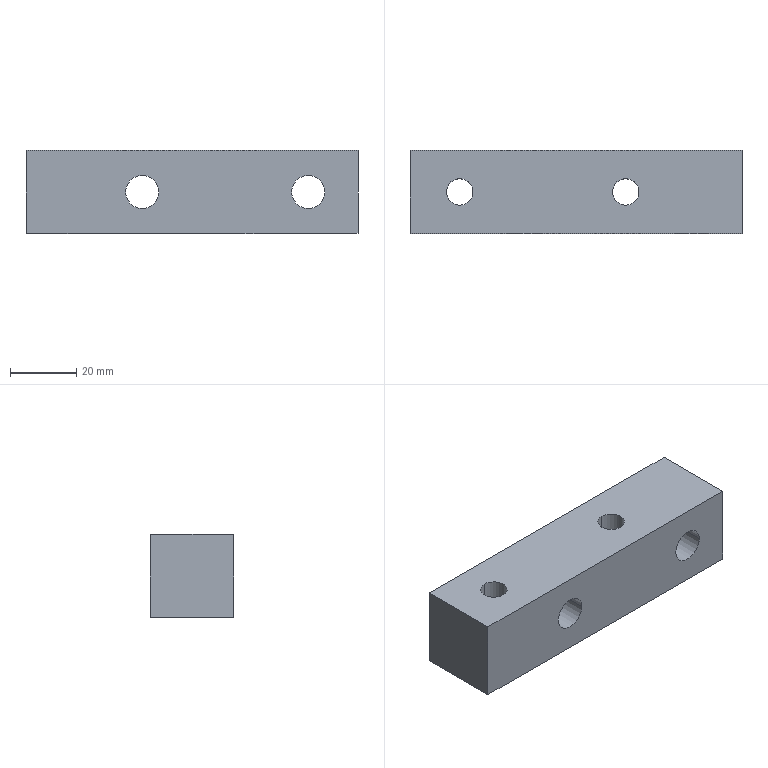Part | STEP file | J453-EBZ05-11-00 | 1 solid | 14 faces | box 100 x 25 x 25 mm | volume 56060 mm3 | cylinder 8 | plane 6 | commonest cylinder face diameters 8 x4 10 x4
STEP:
#1=CARTESIAN_POINT('',(0.,0.,0.));
#2=DIRECTION('',(0.,0.,1.));
#3=DIRECTION('',(1.,0.,0.));
#4=AXIS2_PLACEMENT_3D('',#1,#2,#3);
#5=CARTESIAN_POINT('',(80.,25.,12.5));
#6=VERTEX_POINT('',#5);
#7=CARTESIAN_POINT('',(80.,0.,12.5));
#8=VERTEX_POINT('',#7);
#9=CARTESIAN_POINT('',(80.,25.,12.5));
#10=DIRECTION('',(0.,-1.,0.));
#11=VECTOR('',#10,1.);
#12=LINE('',#9,#11);
#13=CARTESIAN_POINT('',(85.,25.,12.5));
#14=DIRECTION('',(0.,-1.,0.));
#15=DIRECTION('',(-1.,0.,0.));
#16=AXIS2_PLACEMENT_3D('',#13,#14,#15);
#17=CYLINDRICAL_SURFACE('',#16,5.);
#18=CARTESIAN_POINT('',(6.283,0.));
#19=DIRECTION('',(0.,1.));
#20=VECTOR('',#19,1.);
#21=LINE('',#18,#20);
#22=(GEOMETRIC_REPRESENTATION_CONTEXT(2)PARAMETRIC_REPRESENTATION_CONTEXT()REPRESENTATION_CONTEXT('',''));
#23=DEFINITIONAL_REPRESENTATION('',(#21),#22);
#24=PCURVE('',#17,#23);
#25=CARTESIAN_POINT('',(85.,25.,12.5));
#26=DIRECTION('',(0.,-1.,0.));
#27=DIRECTION('',(-1.,0.,0.));
#28=AXIS2_PLACEMENT_3D('',#25,#26,#27);
#29=CYLINDRICAL_SURFACE('',#28,5.);
#30=CARTESIAN_POINT('',(0.,0.));
#31=DIRECTION('',(0.,1.));
#32=VECTOR('',#31,1.);
#33=LINE('',#30,#32);
#34=(GEOMETRIC_REPRESENTATION_CONTEXT(2)PARAMETRIC_REPRESENTATION_CONTEXT()REPRESENTATION_CONTEXT('',''));
#35=DEFINITIONAL_REPRESENTATION('',(#33),#34);
#36=PCURVE('',#29,#35);
#37=SURFACE_CURVE('',#12,(#24,#36),.PCURVE_S1.);
#38=EDGE_CURVE('',#6,#8,#37,.T.);
#39=ORIENTED_EDGE('',*,*,#38,.T.);
#40=CARTESIAN_POINT('',(90.,0.,12.5));
#41=VERTEX_POINT('',#40);
#42=CARTESIAN_POINT('',(85.,0.,12.5));
#43=DIRECTION('',(0.,1.,0.));
#44=DIRECTION('',(1.,0.,0.));
#45=AXIS2_PLACEMENT_3D('',#42,#43,#44);
#46=CIRCLE('',#45,5.);
#47=CARTESIAN_POINT('',(9.425,25.));
#48=DIRECTION('',(-1.,0.));
#49=VECTOR('',#48,1.);
#50=LINE('',#47,#49);
#51=(GEOMETRIC_REPRESENTATION_CONTEXT(2)PARAMETRIC_REPRESENTATION_CONTEXT()REPRESENTATION_CONTEXT('',''));
#52=DEFINITIONAL_REPRESENTATION('',(#50),#51);
#53=PCURVE('',#17,#52);
#54=CARTESIAN_POINT('',(0.,0.,12.5));
#55=DIRECTION('',(0.,-1.,0.));
#56=DIRECTION('',(-1.,0.,0.));
#57=AXIS2_PLACEMENT_3D('',#54,#55,#56);
#58=PLANE('',#57);
#59=CARTESIAN_POINT('',(-90.,0.));
#60=CARTESIAN_POINT('',(-90.,8.66));
#61=CARTESIAN_POINT('',(-82.5,4.33));
#62=CARTESIAN_POINT('',(-75.,0.));
#63=CARTESIAN_POINT('',(-82.5,-4.33));
#64=CARTESIAN_POINT('',(-90.,-8.66));
#65=CARTESIAN_POINT('',(-90.,0.));
#66=(BOUNDED_CURVE()B_SPLINE_CURVE(2,(#59,#60,#61,#62,#63,#64,#65),.UNSPECIFIED.,.T.,.F.)B_SPLINE_CURVE_WITH_KNOTS((1,2,2,2,2,1),(-2.094,0.,2.094,4.189,6.283,8.378),.UNSPECIFIED.)CURVE()GEOMETRIC_REPRESENTATION_ITEM()RATIONAL_B_SPLINE_CURVE((1.,0.5,1.,0.5,1.,0.5,1.))REPRESENTATION_ITEM(''));
#67=(GEOMETRIC_REPRESENTATION_CONTEXT(2)PARAMETRIC_REPRESENTATION_CONTEXT()REPRESENTATION_CONTEXT('',''));
#68=DEFINITIONAL_REPRESENTATION('',(#66),#67);
#69=PCURVE('',#58,#68);
#70=SURFACE_CURVE('',#46,(#53,#69),.PCURVE_S1.);
#71=EDGE_CURVE('',#8,#41,#70,.T.);
#72=ORIENTED_EDGE('',*,*,#71,.T.);
#73=CARTESIAN_POINT('',(90.,25.,12.5));
#74=VERTEX_POINT('',#73);
#75=CARTESIAN_POINT('',(90.,25.,12.5));
#76=DIRECTION('',(0.,-1.,0.));
#77=VECTOR('',#76,1.);
#78=LINE('',#75,#77);
#79=CARTESIAN_POINT('',(3.142,0.));
#80=DIRECTION('',(0.,1.));
#81=VECTOR('',#80,1.);
#82=LINE('',#79,#81);
#83=(GEOMETRIC_REPRESENTATION_CONTEXT(2)PARAMETRIC_REPRESENTATION_CONTEXT()REPRESENTATION_CONTEXT('',''));
#84=DEFINITIONAL_REPRESENTATION('',(#82),#83);
#85=PCURVE('',#17,#84);
#86=CARTESIAN_POINT('',(3.142,0.));
#87=DIRECTION('',(0.,1.));
#88=VECTOR('',#87,1.);
#89=LINE('',#86,#88);
#90=(GEOMETRIC_REPRESENTATION_CONTEXT(2)PARAMETRIC_REPRESENTATION_CONTEXT()REPRESENTATION_CONTEXT('',''));
#91=DEFINITIONAL_REPRESENTATION('',(#89),#90);
#92=PCURVE('',#29,#91);
#93=SURFACE_CURVE('',#78,(#85,#92),.PCURVE_S1.);
#94=EDGE_CURVE('',#74,#41,#93,.T.);
#95=ORIENTED_EDGE('',*,*,#94,.F.);
#96=CARTESIAN_POINT('',(85.,25.,12.5));
#97=DIRECTION('',(0.,-1.,0.));
#98=DIRECTION('',(-1.,0.,0.));
#99=AXIS2_PLACEMENT_3D('',#96,#97,#98);
#100=CIRCLE('',#99,5.);
#101=CARTESIAN_POINT('',(0.,0.));
#102=DIRECTION('',(1.,0.));
#103=VECTOR('',#102,1.);
#104=LINE('',#101,#103);
#105=(GEOMETRIC_REPRESENTATION_CONTEXT(2)PARAMETRIC_REPRESENTATION_CONTEXT()REPRESENTATION_CONTEXT('',''));
#106=DEFINITIONAL_REPRESENTATION('',(#104),#105);
#107=PCURVE('',#17,#106);
#108=CARTESIAN_POINT('',(0.,25.,12.5));
#109=DIRECTION('',(0.,1.,0.));
#110=DIRECTION('',(1.,0.,0.));
#111=AXIS2_PLACEMENT_3D('',#108,#109,#110);
#112=PLANE('',#111);
#113=CARTESIAN_POINT('',(80.,0.));
#114=CARTESIAN_POINT('',(80.,8.66));
#115=CARTESIAN_POINT('',(87.5,4.33));
#116=CARTESIAN_POINT('',(95.,0.));
#117=CARTESIAN_POINT('',(87.5,-4.33));
#118=CARTESIAN_POINT('',(80.,-8.66));
#119=CARTESIAN_POINT('',(80.,0.));
#120=(BOUNDED_CURVE()B_SPLINE_CURVE(2,(#113,#114,#115,#116,#117,#118,#119),.UNSPECIFIED.,.T.,.F.)B_SPLINE_CURVE_WITH_KNOTS((1,2,2,2,2,1),(-2.094,0.,2.094,4.189,6.283,8.378),.UNSPECIFIED.)CURVE()GEOMETRIC_REPRESENTATION_ITEM()RATIONAL_B_SPLINE_CURVE((1.,0.5,1.,0.5,1.,0.5,1.))REPRESENTATION_ITEM(''));
#121=(GEOMETRIC_REPRESENTATION_CONTEXT(2)PARAMETRIC_REPRESENTATION_CONTEXT()REPRESENTATION_CONTEXT('',''));
#122=DEFINITIONAL_REPRESENTATION('',(#120),#121);
#123=PCURVE('',#112,#122);
#124=SURFACE_CURVE('',#100,(#107,#123),.PCURVE_S1.);
#125=EDGE_CURVE('',#74,#6,#124,.T.);
#126=ORIENTED_EDGE('',*,*,#125,.T.);
#127=EDGE_LOOP('',(#39,#72,#95,#126));
#128=FACE_BOUND('',#127,.F.);
#129=ADVANCED_FACE('',(#128),#17,.F.);
#130=CARTESIAN_POINT('',(30.,25.,12.5));
#131=VERTEX_POINT('',#130);
#132=CARTESIAN_POINT('',(30.,0.,12.5));
#133=VERTEX_POINT('',#132);
#134=CARTESIAN_POINT('',(30.,25.,12.5));
#135=DIRECTION('',(0.,-1.,0.));
#136=VECTOR('',#135,1.);
#137=LINE('',#134,#136);
#138=CARTESIAN_POINT('',(35.,25.,12.5));
#139=DIRECTION('',(0.,-1.,0.));
#140=DIRECTION('',(-1.,0.,0.));
#141=AXIS2_PLACEMENT_3D('',#138,#139,#140);
#142=CYLINDRICAL_SURFACE('',#141,5.);
#143=CARTESIAN_POINT('',(6.283,0.));
#144=DIRECTION('',(0.,1.));
#145=VECTOR('',#144,1.);
#146=LINE('',#143,#145);
#147=(GEOMETRIC_REPRESENTATION_CONTEXT(2)PARAMETRIC_REPRESENTATION_CONTEXT()REPRESENTATION_CONTEXT('',''));
#148=DEFINITIONAL_REPRESENTATION('',(#146),#147);
#149=PCURVE('',#142,#148);
#150=CARTESIAN_POINT('',(35.,25.,12.5));
#151=DIRECTION('',(0.,-1.,0.));
#152=DIRECTION('',(-1.,0.,0.));
#153=AXIS2_PLACEMENT_3D('',#150,#151,#152);
#154=CYLINDRICAL_SURFACE('',#153,5.);
#155=CARTESIAN_POINT('',(0.,0.));
#156=DIRECTION('',(0.,1.));
#157=VECTOR('',#156,1.);
#158=LINE('',#155,#157);
#159=(GEOMETRIC_REPRESENTATION_CONTEXT(2)PARAMETRIC_REPRESENTATION_CONTEXT()REPRESENTATION_CONTEXT('',''));
#160=DEFINITIONAL_REPRESENTATION('',(#158),#159);
#161=PCURVE('',#154,#160);
#162=SURFACE_CURVE('',#137,(#149,#161),.PCURVE_S1.);
#163=EDGE_CURVE('',#131,#133,#162,.T.);
#164=ORIENTED_EDGE('',*,*,#163,.T.);
#165=CARTESIAN_POINT('',(40.,0.,12.5));
#166=VERTEX_POINT('',#165);
#167=CARTESIAN_POINT('',(35.,0.,12.5));
#168=DIRECTION('',(0.,1.,0.));
#169=DIRECTION('',(1.,0.,0.));
#170=AXIS2_PLACEMENT_3D('',#167,#168,#169);
#171=CIRCLE('',#170,5.);
#172=CARTESIAN_POINT('',(9.425,25.));
#173=DIRECTION('',(-1.,0.));
#174=VECTOR('',#173,1.);
#175=LINE('',#172,#174);
#176=(GEOMETRIC_REPRESENTATION_CONTEXT(2)PARAMETRIC_REPRESENTATION_CONTEXT()REPRESENTATION_CONTEXT('',''));
#177=DEFINITIONAL_REPRESENTATION('',(#175),#176);
#178=PCURVE('',#142,#177);
#179=CARTESIAN_POINT('',(-40.,0.));
#180=CARTESIAN_POINT('',(-40.,8.66));
#181=CARTESIAN_POINT('',(-32.5,4.33));
#182=CARTESIAN_POINT('',(-25.,0.));
#183=CARTESIAN_POINT('',(-32.5,-4.33));
#184=CARTESIAN_POINT('',(-40.,-8.66));
#185=CARTESIAN_POINT('',(-40.,0.));
#186=(BOUNDED_CURVE()B_SPLINE_CURVE(2,(#179,#180,#181,#182,#183,#184,#185),.UNSPECIFIED.,.T.,.F.)B_SPLINE_CURVE_WITH_KNOTS((1,2,2,2,2,1),(-2.094,0.,2.094,4.189,6.283,8.378),.UNSPECIFIED.)CURVE()GEOMETRIC_REPRESENTATION_ITEM()RATIONAL_B_SPLINE_CURVE((1.,0.5,1.,0.5,1.,0.5,1.))REPRESENTATION_ITEM(''));
#187=(GEOMETRIC_REPRESENTATION_CONTEXT(2)PARAMETRIC_REPRESENTATION_CONTEXT()REPRESENTATION_CONTEXT('',''));
#188=DEFINITIONAL_REPRESENTATION('',(#186),#187);
#189=PCURVE('',#58,#188);
#190=SURFACE_CURVE('',#171,(#178,#189),.PCURVE_S1.);
#191=EDGE_CURVE('',#133,#166,#190,.T.);
#192=ORIENTED_EDGE('',*,*,#191,.T.);
#193=CARTESIAN_POINT('',(40.,25.,12.5));
#194=VERTEX_POINT('',#193);
#195=CARTESIAN_POINT('',(40.,25.,12.5));
#196=DIRECTION('',(0.,-1.,0.));
#197=VECTOR('',#196,1.);
#198=LINE('',#195,#197);
#199=CARTESIAN_POINT('',(3.142,0.));
#200=DIRECTION('',(0.,1.));
#201=VECTOR('',#200,1.);
#202=LINE('',#199,#201);
#203=(GEOMETRIC_REPRESENTATION_CONTEXT(2)PARAMETRIC_REPRESENTATION_CONTEXT()REPRESENTATION_CONTEXT('',''));
#204=DEFINITIONAL_REPRESENTATION('',(#202),#203);
#205=PCURVE('',#142,#204);
#206=CARTESIAN_POINT('',(3.142,0.));
#207=DIRECTION('',(0.,1.));
#208=VECTOR('',#207,1.);
#209=LINE('',#206,#208);
#210=(GEOMETRIC_REPRESENTATION_CONTEXT(2)PARAMETRIC_REPRESENTATION_CONTEXT()REPRESENTATION_CONTEXT('',''));
#211=DEFINITIONAL_REPRESENTATION('',(#209),#210);
#212=PCURVE('',#154,#211);
#213=SURFACE_CURVE('',#198,(#205,#212),.PCURVE_S1.);
#214=EDGE_CURVE('',#194,#166,#213,.T.);
#215=ORIENTED_EDGE('',*,*,#214,.F.);
#216=CARTESIAN_POINT('',(35.,25.,12.5));
#217=DIRECTION('',(0.,-1.,0.));
#218=DIRECTION('',(-1.,0.,0.));
#219=AXIS2_PLACEMENT_3D('',#216,#217,#218);
#220=CIRCLE('',#219,5.);
#221=CARTESIAN_POINT('',(0.,0.));
#222=DIRECTION('',(1.,0.));
#223=VECTOR('',#222,1.);
#224=LINE('',#221,#223);
#225=(GEOMETRIC_REPRESENTATION_CONTEXT(2)PARAMETRIC_REPRESENTATION_CONTEXT()REPRESENTATION_CONTEXT('',''));
#226=DEFINITIONAL_REPRESENTATION('',(#224),#225);
#227=PCURVE('',#142,#226);
#228=CARTESIAN_POINT('',(30.,0.));
#229=CARTESIAN_POINT('',(30.,8.66));
#230=CARTESIAN_POINT('',(37.5,4.33));
#231=CARTESIAN_POINT('',(45.,0.));
#232=CARTESIAN_POINT('',(37.5,-4.33));
#233=CARTESIAN_POINT('',(30.,-8.66));
#234=CARTESIAN_POINT('',(30.,0.));
#235=(BOUNDED_CURVE()B_SPLINE_CURVE(2,(#228,#229,#230,#231,#232,#233,#234),.UNSPECIFIED.,.T.,.F.)B_SPLINE_CURVE_WITH_KNOTS((1,2,2,2,2,1),(-2.094,0.,2.094,4.189,6.283,8.378),.UNSPECIFIED.)CURVE()GEOMETRIC_REPRESENTATION_ITEM()RATIONAL_B_SPLINE_CURVE((1.,0.5,1.,0.5,1.,0.5,1.))REPRESENTATION_ITEM(''));
#236=(GEOMETRIC_REPRESENTATION_CONTEXT(2)PARAMETRIC_REPRESENTATION_CONTEXT()REPRESENTATION_CONTEXT('',''));
#237=DEFINITIONAL_REPRESENTATION('',(#235),#236);
#238=PCURVE('',#112,#237);
#239=SURFACE_CURVE('',#220,(#227,#238),.PCURVE_S1.);
#240=EDGE_CURVE('',#194,#131,#239,.T.);
#241=ORIENTED_EDGE('',*,*,#240,.T.);
#242=EDGE_LOOP('',(#164,#192,#215,#241));
#243=FACE_BOUND('',#242,.F.);
#244=ADVANCED_FACE('',(#243),#142,.F.);
#245=CARTESIAN_POINT('',(65.,8.5,0.));
#246=VERTEX_POINT('',#245);
#247=CARTESIAN_POINT('',(65.,8.5,25.));
#248=VERTEX_POINT('',#247);
#249=CARTESIAN_POINT('',(65.,8.5,0.));
#250=DIRECTION('',(0.,0.,1.));
#251=VECTOR('',#250,1.);
#252=LINE('',#249,#251);
#253=CARTESIAN_POINT('',(65.,12.5,0.));
#254=DIRECTION('',(0.,0.,1.));
#255=DIRECTION('',(0.,-1.,0.));
#256=AXIS2_PLACEMENT_3D('',#253,#254,#255);
#257=CYLINDRICAL_SURFACE('',#256,4.);
#258=CARTESIAN_POINT('',(6.283,0.));
#259=DIRECTION('',(0.,1.));
#260=VECTOR('',#259,1.);
#261=LINE('',#258,#260);
#262=(GEOMETRIC_REPRESENTATION_CONTEXT(2)PARAMETRIC_REPRESENTATION_CONTEXT()REPRESENTATION_CONTEXT('',''));
#263=DEFINITIONAL_REPRESENTATION('',(#261),#262);
#264=PCURVE('',#257,#263);
#265=CARTESIAN_POINT('',(65.,12.5,0.));
#266=DIRECTION('',(0.,0.,1.));
#267=DIRECTION('',(0.,-1.,0.));
#268=AXIS2_PLACEMENT_3D('',#265,#266,#267);
#269=CYLINDRICAL_SURFACE('',#268,4.);
#270=CARTESIAN_POINT('',(0.,0.));
#271=DIRECTION('',(0.,1.));
#272=VECTOR('',#271,1.);
#273=LINE('',#270,#272);
#274=(GEOMETRIC_REPRESENTATION_CONTEXT(2)PARAMETRIC_REPRESENTATION_CONTEXT()REPRESENTATION_CONTEXT('',''));
#275=DEFINITIONAL_REPRESENTATION('',(#273),#274);
#276=PCURVE('',#269,#275);
#277=SURFACE_CURVE('',#252,(#264,#276),.PCURVE_S1.);
#278=EDGE_CURVE('',#246,#248,#277,.T.);
#279=ORIENTED_EDGE('',*,*,#278,.T.);
#280=CARTESIAN_POINT('',(65.,16.5,25.));
#281=VERTEX_POINT('',#280);
#282=CARTESIAN_POINT('',(65.,12.5,25.));
#283=DIRECTION('',(0.,0.,-1.));
#284=DIRECTION('',(0.,1.,0.));
#285=AXIS2_PLACEMENT_3D('',#282,#283,#284);
#286=CIRCLE('',#285,4.);
#287=CARTESIAN_POINT('',(9.425,25.));
#288=DIRECTION('',(-1.,0.));
#289=VECTOR('',#288,1.);
#290=LINE('',#287,#289);
#291=(GEOMETRIC_REPRESENTATION_CONTEXT(2)PARAMETRIC_REPRESENTATION_CONTEXT()REPRESENTATION_CONTEXT('',''));
#292=DEFINITIONAL_REPRESENTATION('',(#290),#291);
#293=PCURVE('',#257,#292);
#294=CARTESIAN_POINT('',(0.,12.5,25.));
#295=DIRECTION('',(0.,0.,1.));
#296=DIRECTION('',(1.,0.,0.));
#297=AXIS2_PLACEMENT_3D('',#294,#295,#296);
#298=PLANE('',#297);
#299=CARTESIAN_POINT('',(65.,4.));
#300=CARTESIAN_POINT('',(71.928,4.));
#301=CARTESIAN_POINT('',(68.464,-2.));
#302=CARTESIAN_POINT('',(65.,-8.));
#303=CARTESIAN_POINT('',(61.536,-2.));
#304=CARTESIAN_POINT('',(58.072,4.));
#305=CARTESIAN_POINT('',(65.,4.));
#306=(BOUNDED_CURVE()B_SPLINE_CURVE(2,(#299,#300,#301,#302,#303,#304,#305),.UNSPECIFIED.,.T.,.F.)B_SPLINE_CURVE_WITH_KNOTS((1,2,2,2,2,1),(-2.094,0.,2.094,4.189,6.283,8.378),.UNSPECIFIED.)CURVE()GEOMETRIC_REPRESENTATION_ITEM()RATIONAL_B_SPLINE_CURVE((1.,0.5,1.,0.5,1.,0.5,1.))REPRESENTATION_ITEM(''));
#307=(GEOMETRIC_REPRESENTATION_CONTEXT(2)PARAMETRIC_REPRESENTATION_CONTEXT()REPRESENTATION_CONTEXT('',''));
#308=DEFINITIONAL_REPRESENTATION('',(#306),#307);
#309=PCURVE('',#298,#308);
#310=SURFACE_CURVE('',#286,(#293,#309),.PCURVE_S1.);
#311=EDGE_CURVE('',#248,#281,#310,.T.);
#312=ORIENTED_EDGE('',*,*,#311,.T.);
#313=CARTESIAN_POINT('',(65.,16.5,0.));
#314=VERTEX_POINT('',#313);
#315=CARTESIAN_POINT('',(65.,16.5,0.));
#316=DIRECTION('',(0.,0.,1.));
#317=VECTOR('',#316,1.);
#318=LINE('',#315,#317);
#319=CARTESIAN_POINT('',(3.142,0.));
#320=DIRECTION('',(0.,1.));
#321=VECTOR('',#320,1.);
#322=LINE('',#319,#321);
#323=(GEOMETRIC_REPRESENTATION_CONTEXT(2)PARAMETRIC_REPRESENTATION_CONTEXT()REPRESENTATION_CONTEXT('',''));
#324=DEFINITIONAL_REPRESENTATION('',(#322),#323);
#325=PCURVE('',#257,#324);
#326=CARTESIAN_POINT('',(3.142,0.));
#327=DIRECTION('',(0.,1.));
#328=VECTOR('',#327,1.);
#329=LINE('',#326,#328);
#330=(GEOMETRIC_REPRESENTATION_CONTEXT(2)PARAMETRIC_REPRESENTATION_CONTEXT()REPRESENTATION_CONTEXT('',''));
#331=DEFINITIONAL_REPRESENTATION('',(#329),#330);
#332=PCURVE('',#269,#331);
#333=SURFACE_CURVE('',#318,(#325,#332),.PCURVE_S1.);
#334=EDGE_CURVE('',#314,#281,#333,.T.);
#335=ORIENTED_EDGE('',*,*,#334,.F.);
#336=CARTESIAN_POINT('',(65.,12.5,0.));
#337=DIRECTION('',(0.,0.,1.));
#338=DIRECTION('',(0.,-1.,0.));
#339=AXIS2_PLACEMENT_3D('',#336,#337,#338);
#340=CIRCLE('',#339,4.);
#341=CARTESIAN_POINT('',(0.,0.));
#342=DIRECTION('',(1.,0.));
#343=VECTOR('',#342,1.);
#344=LINE('',#341,#343);
#345=(GEOMETRIC_REPRESENTATION_CONTEXT(2)PARAMETRIC_REPRESENTATION_CONTEXT()REPRESENTATION_CONTEXT('',''));
#346=DEFINITIONAL_REPRESENTATION('',(#344),#345);
#347=PCURVE('',#257,#346);
#348=CARTESIAN_POINT('',(0.,12.5,0.));
#349=DIRECTION('',(0.,0.,-1.));
#350=DIRECTION('',(-1.,0.,0.));
#351=AXIS2_PLACEMENT_3D('',#348,#349,#350);
#352=PLANE('',#351);
#353=CARTESIAN_POINT('',(-65.,-4.));
#354=CARTESIAN_POINT('',(-71.928,-4.));
#355=CARTESIAN_POINT('',(-68.464,2.));
#356=CARTESIAN_POINT('',(-65.,8.));
#357=CARTESIAN_POINT('',(-61.536,2.));
#358=CARTESIAN_POINT('',(-58.072,-4.));
#359=CARTESIAN_POINT('',(-65.,-4.));
#360=(BOUNDED_CURVE()B_SPLINE_CURVE(2,(#353,#354,#355,#356,#357,#358,#359),.UNSPECIFIED.,.T.,.F.)B_SPLINE_CURVE_WITH_KNOTS((1,2,2,2,2,1),(-2.094,0.,2.094,4.189,6.283,8.378),.UNSPECIFIED.)CURVE()GEOMETRIC_REPRESENTATION_ITEM()RATIONAL_B_SPLINE_CURVE((1.,0.5,1.,0.5,1.,0.5,1.))REPRESENTATION_ITEM(''));
#361=(GEOMETRIC_REPRESENTATION_CONTEXT(2)PARAMETRIC_REPRESENTATION_CONTEXT()REPRESENTATION_CONTEXT('',''));
#362=DEFINITIONAL_REPRESENTATION('',(#360),#361);
#363=PCURVE('',#352,#362);
#364=SURFACE_CURVE('',#340,(#347,#363),.PCURVE_S1.);
#365=EDGE_CURVE('',#314,#246,#364,.T.);
#366=ORIENTED_EDGE('',*,*,#365,.T.);
#367=EDGE_LOOP('',(#279,#312,#335,#366));
#368=FACE_BOUND('',#367,.F.);
#369=ADVANCED_FACE('',(#368),#257,.F.);
#370=CARTESIAN_POINT('',(15.,8.5,0.));
#371=VERTEX_POINT('',#370);
#372=CARTESIAN_POINT('',(15.,8.5,25.));
#373=VERTEX_POINT('',#372);
#374=CARTESIAN_POINT('',(15.,8.5,0.));
#375=DIRECTION('',(0.,0.,1.));
#376=VECTOR('',#375,1.);
#377=LINE('',#374,#376);
#378=CARTESIAN_POINT('',(15.,12.5,0.));
#379=DIRECTION('',(0.,0.,1.));
#380=DIRECTION('',(0.,-1.,0.));
#381=AXIS2_PLACEMENT_3D('',#378,#379,#380);
#382=CYLINDRICAL_SURFACE('',#381,4.);
#383=CARTESIAN_POINT('',(6.283,0.));
#384=DIRECTION('',(0.,1.));
#385=VECTOR('',#384,1.);
#386=LINE('',#383,#385);
#387=(GEOMETRIC_REPRESENTATION_CONTEXT(2)PARAMETRIC_REPRESENTATION_CONTEXT()REPRESENTATION_CONTEXT('',''));
#388=DEFINITIONAL_REPRESENTATION('',(#386),#387);
#389=PCURVE('',#382,#388);
#390=CARTESIAN_POINT('',(15.,12.5,0.));
#391=DIRECTION('',(0.,0.,1.));
#392=DIRECTION('',(0.,-1.,0.));
#393=AXIS2_PLACEMENT_3D('',#390,#391,#392);
#394=CYLINDRICAL_SURFACE('',#393,4.);
#395=CARTESIAN_POINT('',(0.,0.));
#396=DIRECTION('',(0.,1.));
#397=VECTOR('',#396,1.);
#398=LINE('',#395,#397);
#399=(GEOMETRIC_REPRESENTATION_CONTEXT(2)PARAMETRIC_REPRESENTATION_CONTEXT()REPRESENTATION_CONTEXT('',''));
#400=DEFINITIONAL_REPRESENTATION('',(#398),#399);
#401=PCURVE('',#394,#400);
#402=SURFACE_CURVE('',#377,(#389,#401),.PCURVE_S1.);
#403=EDGE_CURVE('',#371,#373,#402,.T.);
#404=ORIENTED_EDGE('',*,*,#403,.T.);
#405=CARTESIAN_POINT('',(15.,16.5,25.));
#406=VERTEX_POINT('',#405);
#407=CARTESIAN_POINT('',(15.,12.5,25.));
#408=DIRECTION('',(0.,0.,-1.));
#409=DIRECTION('',(0.,1.,0.));
#410=AXIS2_PLACEMENT_3D('',#407,#408,#409);
#411=CIRCLE('',#410,4.);
#412=CARTESIAN_POINT('',(9.425,25.));
#413=DIRECTION('',(-1.,0.));
#414=VECTOR('',#413,1.);
#415=LINE('',#412,#414);
#416=(GEOMETRIC_REPRESENTATION_CONTEXT(2)PARAMETRIC_REPRESENTATION_CONTEXT()REPRESENTATION_CONTEXT('',''));
#417=DEFINITIONAL_REPRESENTATION('',(#415),#416);
#418=PCURVE('',#382,#417);
#419=CARTESIAN_POINT('',(15.,4.));
#420=CARTESIAN_POINT('',(21.928,4.));
#421=CARTESIAN_POINT('',(18.464,-2.));
#422=CARTESIAN_POINT('',(15.,-8.));
#423=CARTESIAN_POINT('',(11.536,-2.));
#424=CARTESIAN_POINT('',(8.072,4.));
#425=CARTESIAN_POINT('',(15.,4.));
#426=(BOUNDED_CURVE()B_SPLINE_CURVE(2,(#419,#420,#421,#422,#423,#424,#425),.UNSPECIFIED.,.T.,.F.)B_SPLINE_CURVE_WITH_KNOTS((1,2,2,2,2,1),(-2.094,0.,2.094,4.189,6.283,8.378),.UNSPECIFIED.)CURVE()GEOMETRIC_REPRESENTATION_ITEM()RATIONAL_B_SPLINE_CURVE((1.,0.5,1.,0.5,1.,0.5,1.))REPRESENTATION_ITEM(''));
#427=(GEOMETRIC_REPRESENTATION_CONTEXT(2)PARAMETRIC_REPRESENTATION_CONTEXT()REPRESENTATION_CONTEXT('',''));
#428=DEFINITIONAL_REPRESENTATION('',(#426),#427);
#429=PCURVE('',#298,#428);
#430=SURFACE_CURVE('',#411,(#418,#429),.PCURVE_S1.);
#431=EDGE_CURVE('',#373,#406,#430,.T.);
#432=ORIENTED_EDGE('',*,*,#431,.T.);
#433=CARTESIAN_POINT('',(15.,16.5,0.));
#434=VERTEX_POINT('',#433);
#435=CARTESIAN_POINT('',(15.,16.5,0.));
#436=DIRECTION('',(0.,0.,1.));
#437=VECTOR('',#436,1.);
#438=LINE('',#435,#437);
#439=CARTESIAN_POINT('',(3.142,0.));
#440=DIRECTION('',(0.,1.));
#441=VECTOR('',#440,1.);
#442=LINE('',#439,#441);
#443=(GEOMETRIC_REPRESENTATION_CONTEXT(2)PARAMETRIC_REPRESENTATION_CONTEXT()REPRESENTATION_CONTEXT('',''));
#444=DEFINITIONAL_REPRESENTATION('',(#442),#443);
#445=PCURVE('',#382,#444);
#446=CARTESIAN_POINT('',(3.142,0.));
#447=DIRECTION('',(0.,1.));
#448=VECTOR('',#447,1.);
#449=LINE('',#446,#448);
#450=(GEOMETRIC_REPRESENTATION_CONTEXT(2)PARAMETRIC_REPRESENTATION_CONTEXT()REPRESENTATION_CONTEXT('',''));
#451=DEFINITIONAL_REPRESENTATION('',(#449),#450);
#452=PCURVE('',#394,#451);
#453=SURFACE_CURVE('',#438,(#445,#452),.PCURVE_S1.);
#454=EDGE_CURVE('',#434,#406,#453,.T.);
#455=ORIENTED_EDGE('',*,*,#454,.F.);
#456=CARTESIAN_POINT('',(15.,12.5,0.));
#457=DIRECTION('',(0.,0.,1.));
#458=DIRECTION('',(0.,-1.,0.));
#459=AXIS2_PLACEMENT_3D('',#456,#457,#458);
#460=CIRCLE('',#459,4.);
#461=CARTESIAN_POINT('',(0.,0.));
#462=DIRECTION('',(1.,0.));
#463=VECTOR('',#462,1.);
#464=LINE('',#461,#463);
#465=(GEOMETRIC_REPRESENTATION_CONTEXT(2)PARAMETRIC_REPRESENTATION_CONTEXT()REPRESENTATION_CONTEXT('',''));
#466=DEFINITIONAL_REPRESENTATION('',(#464),#465);
#467=PCURVE('',#382,#466);
#468=CARTESIAN_POINT('',(-15.,-4.));
#469=CARTESIAN_POINT('',(-21.928,-4.));
#470=CARTESIAN_POINT('',(-18.464,2.));
#471=CARTESIAN_POINT('',(-15.,8.));
#472=CARTESIAN_POINT('',(-11.536,2.));
#473=CARTESIAN_POINT('',(-8.072,-4.));
#474=CARTESIAN_POINT('',(-15.,-4.));
#475=(BOUNDED_CURVE()B_SPLINE_CURVE(2,(#468,#469,#470,#471,#472,#473,#474),.UNSPECIFIED.,.T.,.F.)B_SPLINE_CURVE_WITH_KNOTS((1,2,2,2,2,1),(-2.094,0.,2.094,4.189,6.283,8.378),.UNSPECIFIED.)CURVE()GEOMETRIC_REPRESENTATION_ITEM()RATIONAL_B_SPLINE_CURVE((1.,0.5,1.,0.5,1.,0.5,1.))REPRESENTATION_ITEM(''));
#476=(GEOMETRIC_REPRESENTATION_CONTEXT(2)PARAMETRIC_REPRESENTATION_CONTEXT()REPRESENTATION_CONTEXT('',''));
#477=DEFINITIONAL_REPRESENTATION('',(#475),#476);
#478=PCURVE('',#352,#477);
#479=SURFACE_CURVE('',#460,(#467,#478),.PCURVE_S1.);
#480=EDGE_CURVE('',#434,#371,#479,.T.);
#481=ORIENTED_EDGE('',*,*,#480,.T.);
#482=EDGE_LOOP('',(#404,#432,#455,#481));
#483=FACE_BOUND('',#482,.F.);
#484=ADVANCED_FACE('',(#483),#382,.F.);
#485=CARTESIAN_POINT('',(100.,0.,0.));
#486=VERTEX_POINT('',#485);
#487=CARTESIAN_POINT('',(100.,0.,25.));
#488=VERTEX_POINT('',#487);
#489=CARTESIAN_POINT('',(100.,0.,12.5));
#490=DIRECTION('',(0.,0.,1.));
#491=VECTOR('',#490,1.);
#492=LINE('',#489,#491);
#493=CARTESIAN_POINT('',(100.,12.5,12.5));
#494=DIRECTION('',(1.,0.,0.));
#495=DIRECTION('',(0.,0.,-1.));
#496=AXIS2_PLACEMENT_3D('',#493,#494,#495);
#497=PLANE('',#496);
#498=CARTESIAN_POINT('',(0.,-12.5));
#499=DIRECTION('',(-1.,0.));
#500=VECTOR('',#499,1.);
#501=LINE('',#498,#500);
#502=(GEOMETRIC_REPRESENTATION_CONTEXT(2)PARAMETRIC_REPRESENTATION_CONTEXT()REPRESENTATION_CONTEXT('',''));
#503=DEFINITIONAL_REPRESENTATION('',(#501),#502);
#504=PCURVE('',#497,#503);
#505=CARTESIAN_POINT('',(-100.,0.));
#506=DIRECTION('',(0.,-1.));
#507=VECTOR('',#506,1.);
#508=LINE('',#505,#507);
#509=(GEOMETRIC_REPRESENTATION_CONTEXT(2)PARAMETRIC_REPRESENTATION_CONTEXT()REPRESENTATION_CONTEXT('',''));
#510=DEFINITIONAL_REPRESENTATION('',(#508),#509);
#511=PCURVE('',#58,#510);
#512=SURFACE_CURVE('',#492,(#504,#511),.PCURVE_S1.);
#513=EDGE_CURVE('',#486,#488,#512,.T.);
#514=ORIENTED_EDGE('',*,*,#513,.F.);
#515=CARTESIAN_POINT('',(100.,25.,0.));
#516=VERTEX_POINT('',#515);
#517=CARTESIAN_POINT('',(100.,12.5,0.));
#518=DIRECTION('',(0.,-1.,0.));
#519=VECTOR('',#518,1.);
#520=LINE('',#517,#519);
#521=CARTESIAN_POINT('',(12.5,0.));
#522=DIRECTION('',(0.,-1.));
#523=VECTOR('',#522,1.);
#524=LINE('',#521,#523);
#525=(GEOMETRIC_REPRESENTATION_CONTEXT(2)PARAMETRIC_REPRESENTATION_CONTEXT()REPRESENTATION_CONTEXT('',''));
#526=DEFINITIONAL_REPRESENTATION('',(#524),#525);
#527=PCURVE('',#497,#526);
#528=CARTESIAN_POINT('',(-100.,0.));
#529=DIRECTION('',(0.,-1.));
#530=VECTOR('',#529,1.);
#531=LINE('',#528,#530);
#532=(GEOMETRIC_REPRESENTATION_CONTEXT(2)PARAMETRIC_REPRESENTATION_CONTEXT()REPRESENTATION_CONTEXT('',''));
#533=DEFINITIONAL_REPRESENTATION('',(#531),#532);
#534=PCURVE('',#352,#533);
#535=SURFACE_CURVE('',#520,(#527,#534),.PCURVE_S1.);
#536=EDGE_CURVE('',#516,#486,#535,.T.);
#537=ORIENTED_EDGE('',*,*,#536,.F.);
#538=CARTESIAN_POINT('',(100.,25.,25.));
#539=VERTEX_POINT('',#538);
#540=CARTESIAN_POINT('',(100.,25.,12.5));
#541=DIRECTION('',(0.,0.,-1.));
#542=VECTOR('',#541,1.);
#543=LINE('',#540,#542);
#544=CARTESIAN_POINT('',(0.,12.5));
#545=DIRECTION('',(1.,0.));
#546=VECTOR('',#545,1.);
#547=LINE('',#544,#546);
#548=(GEOMETRIC_REPRESENTATION_CONTEXT(2)PARAMETRIC_REPRESENTATION_CONTEXT()REPRESENTATION_CONTEXT('',''));
#549=DEFINITIONAL_REPRESENTATION('',(#547),#548);
#550=PCURVE('',#497,#549);
#551=CARTESIAN_POINT('',(100.,0.));
#552=DIRECTION('',(0.,1.));
#553=VECTOR('',#552,1.);
#554=LINE('',#551,#553);
#555=(GEOMETRIC_REPRESENTATION_CONTEXT(2)PARAMETRIC_REPRESENTATION_CONTEXT()REPRESENTATION_CONTEXT('',''));
#556=DEFINITIONAL_REPRESENTATION('',(#554),#555);
#557=PCURVE('',#112,#556);
#558=SURFACE_CURVE('',#543,(#550,#557),.PCURVE_S1.);
#559=EDGE_CURVE('',#539,#516,#558,.T.);
#560=ORIENTED_EDGE('',*,*,#559,.F.);
#561=CARTESIAN_POINT('',(100.,12.5,25.));
#562=DIRECTION('',(0.,1.,0.));
#563=VECTOR('',#562,1.);
#564=LINE('',#561,#563);
#565=CARTESIAN_POINT('',(-12.5,0.));
#566=DIRECTION('',(0.,1.));
#567=VECTOR('',#566,1.);
#568=LINE('',#565,#567);
#569=(GEOMETRIC_REPRESENTATION_CONTEXT(2)PARAMETRIC_REPRESENTATION_CONTEXT()REPRESENTATION_CONTEXT('',''));
#570=DEFINITIONAL_REPRESENTATION('',(#568),#569);
#571=PCURVE('',#497,#570);
#572=CARTESIAN_POINT('',(100.,0.));
#573=DIRECTION('',(0.,1.));
#574=VECTOR('',#573,1.);
#575=LINE('',#572,#574);
#576=(GEOMETRIC_REPRESENTATION_CONTEXT(2)PARAMETRIC_REPRESENTATION_CONTEXT()REPRESENTATION_CONTEXT('',''));
#577=DEFINITIONAL_REPRESENTATION('',(#575),#576);
#578=PCURVE('',#298,#577);
#579=SURFACE_CURVE('',#564,(#571,#578),.PCURVE_S1.);
#580=EDGE_CURVE('',#488,#539,#579,.T.);
#581=ORIENTED_EDGE('',*,*,#580,.F.);
#582=EDGE_LOOP('',(#514,#537,#560,#581));
#583=FACE_BOUND('',#582,.T.);
#584=ADVANCED_FACE('',(#583),#497,.T.);
#585=ORIENTED_EDGE('',*,*,#71,.T.);
#586=CARTESIAN_POINT('',(85.,0.,12.5));
#587=DIRECTION('',(0.,1.,0.));
#588=DIRECTION('',(1.,0.,0.));
#589=AXIS2_PLACEMENT_3D('',#586,#587,#588);
#590=CIRCLE('',#589,5.);
#591=CARTESIAN_POINT('',(-90.,0.));
#592=CARTESIAN_POINT('',(-90.,8.66));
#593=CARTESIAN_POINT('',(-82.5,4.33));
#594=CARTESIAN_POINT('',(-75.,0.));
#595=CARTESIAN_POINT('',(-82.5,-4.33));
#596=CARTESIAN_POINT('',(-90.,-8.66));
#597=CARTESIAN_POINT('',(-90.,0.));
#598=(BOUNDED_CURVE()B_SPLINE_CURVE(2,(#591,#592,#593,#594,#595,#596,#597),.UNSPECIFIED.,.T.,.F.)B_SPLINE_CURVE_WITH_KNOTS((1,2,2,2,2,1),(-2.094,0.,2.094,4.189,6.283,8.378),.UNSPECIFIED.)CURVE()GEOMETRIC_REPRESENTATION_ITEM()RATIONAL_B_SPLINE_CURVE((1.,0.5,1.,0.5,1.,0.5,1.))REPRESENTATION_ITEM(''));
#599=(GEOMETRIC_REPRESENTATION_CONTEXT(2)PARAMETRIC_REPRESENTATION_CONTEXT()REPRESENTATION_CONTEXT('',''));
#600=DEFINITIONAL_REPRESENTATION('',(#598),#599);
#601=PCURVE('',#58,#600);
#602=CARTESIAN_POINT('',(3.142,25.));
#603=DIRECTION('',(-1.,0.));
#604=VECTOR('',#603,1.);
#605=LINE('',#602,#604);
#606=(GEOMETRIC_REPRESENTATION_CONTEXT(2)PARAMETRIC_REPRESENTATION_CONTEXT()REPRESENTATION_CONTEXT('',''));
#607=DEFINITIONAL_REPRESENTATION('',(#605),#606);
#608=PCURVE('',#29,#607);
#609=SURFACE_CURVE('',#590,(#601,#608),.PCURVE_S1.);
#610=EDGE_CURVE('',#41,#8,#609,.T.);
#611=ORIENTED_EDGE('',*,*,#610,.T.);
#612=EDGE_LOOP('',(#585,#611));
#613=FACE_BOUND('',#612,.T.);
#614=ORIENTED_EDGE('',*,*,#191,.T.);
#615=CARTESIAN_POINT('',(35.,0.,12.5));
#616=DIRECTION('',(0.,1.,0.));
#617=DIRECTION('',(1.,0.,0.));
#618=AXIS2_PLACEMENT_3D('',#615,#616,#617);
#619=CIRCLE('',#618,5.);
#620=CARTESIAN_POINT('',(-40.,0.));
#621=CARTESIAN_POINT('',(-40.,8.66));
#622=CARTESIAN_POINT('',(-32.5,4.33));
#623=CARTESIAN_POINT('',(-25.,0.));
#624=CARTESIAN_POINT('',(-32.5,-4.33));
#625=CARTESIAN_POINT('',(-40.,-8.66));
#626=CARTESIAN_POINT('',(-40.,0.));
#627=(BOUNDED_CURVE()B_SPLINE_CURVE(2,(#620,#621,#622,#623,#624,#625,#626),.UNSPECIFIED.,.T.,.F.)B_SPLINE_CURVE_WITH_KNOTS((1,2,2,2,2,1),(-2.094,0.,2.094,4.189,6.283,8.378),.UNSPECIFIED.)CURVE()GEOMETRIC_REPRESENTATION_ITEM()RATIONAL_B_SPLINE_CURVE((1.,0.5,1.,0.5,1.,0.5,1.))REPRESENTATION_ITEM(''));
#628=(GEOMETRIC_REPRESENTATION_CONTEXT(2)PARAMETRIC_REPRESENTATION_CONTEXT()REPRESENTATION_CONTEXT('',''));
#629=DEFINITIONAL_REPRESENTATION('',(#627),#628);
#630=PCURVE('',#58,#629);
#631=CARTESIAN_POINT('',(3.142,25.));
#632=DIRECTION('',(-1.,0.));
#633=VECTOR('',#632,1.);
#634=LINE('',#631,#633);
#635=(GEOMETRIC_REPRESENTATION_CONTEXT(2)PARAMETRIC_REPRESENTATION_CONTEXT()REPRESENTATION_CONTEXT('',''));
#636=DEFINITIONAL_REPRESENTATION('',(#634),#635);
#637=PCURVE('',#154,#636);
#638=SURFACE_CURVE('',#619,(#630,#637),.PCURVE_S1.);
#639=EDGE_CURVE('',#166,#133,#638,.T.);
#640=ORIENTED_EDGE('',*,*,#639,.T.);
#641=EDGE_LOOP('',(#614,#640));
#642=FACE_BOUND('',#641,.T.);
#643=CARTESIAN_POINT('',(0.,0.,0.));
#644=VERTEX_POINT('',#643);
#645=CARTESIAN_POINT('',(0.,0.,0.));
#646=DIRECTION('',(1.,0.,0.));
#647=VECTOR('',#646,1.);
#648=LINE('',#645,#647);
#649=CARTESIAN_POINT('',(0.,12.5));
#650=DIRECTION('',(-1.,0.));
#651=VECTOR('',#650,1.);
#652=LINE('',#649,#651);
#653=(GEOMETRIC_REPRESENTATION_CONTEXT(2)PARAMETRIC_REPRESENTATION_CONTEXT()REPRESENTATION_CONTEXT('',''));
#654=DEFINITIONAL_REPRESENTATION('',(#652),#653);
#655=PCURVE('',#58,#654);
#656=CARTESIAN_POINT('',(0.,-12.5));
#657=DIRECTION('',(-1.,0.));
#658=VECTOR('',#657,1.);
#659=LINE('',#656,#658);
#660=(GEOMETRIC_REPRESENTATION_CONTEXT(2)PARAMETRIC_REPRESENTATION_CONTEXT()REPRESENTATION_CONTEXT('',''));
#661=DEFINITIONAL_REPRESENTATION('',(#659),#660);
#662=PCURVE('',#352,#661);
#663=SURFACE_CURVE('',#648,(#655,#662),.PCURVE_S1.);
#664=EDGE_CURVE('',#644,#486,#663,.T.);
#665=ORIENTED_EDGE('',*,*,#664,.T.);
#666=ORIENTED_EDGE('',*,*,#513,.T.);
#667=CARTESIAN_POINT('',(0.,0.,25.));
#668=VERTEX_POINT('',#667);
#669=CARTESIAN_POINT('',(0.,0.,25.));
#670=DIRECTION('',(1.,0.,0.));
#671=VECTOR('',#670,1.);
#672=LINE('',#669,#671);
#673=CARTESIAN_POINT('',(0.,-12.5));
#674=DIRECTION('',(-1.,0.));
#675=VECTOR('',#674,1.);
#676=LINE('',#673,#675);
#677=(GEOMETRIC_REPRESENTATION_CONTEXT(2)PARAMETRIC_REPRESENTATION_CONTEXT()REPRESENTATION_CONTEXT('',''));
#678=DEFINITIONAL_REPRESENTATION('',(#676),#677);
#679=PCURVE('',#58,#678);
#680=CARTESIAN_POINT('',(0.,-12.5));
#681=DIRECTION('',(1.,0.));
#682=VECTOR('',#681,1.);
#683=LINE('',#680,#682);
#684=(GEOMETRIC_REPRESENTATION_CONTEXT(2)PARAMETRIC_REPRESENTATION_CONTEXT()REPRESENTATION_CONTEXT('',''));
#685=DEFINITIONAL_REPRESENTATION('',(#683),#684);
#686=PCURVE('',#298,#685);
#687=SURFACE_CURVE('',#672,(#679,#686),.PCURVE_S1.);
#688=EDGE_CURVE('',#668,#488,#687,.T.);
#689=ORIENTED_EDGE('',*,*,#688,.F.);
#690=CARTESIAN_POINT('',(0.,0.,12.5));
#691=DIRECTION('',(0.,0.,-1.));
#692=VECTOR('',#691,1.);
#693=LINE('',#690,#692);
#694=CARTESIAN_POINT('',(0.,0.));
#695=DIRECTION('',(0.,1.));
#696=VECTOR('',#695,1.);
#697=LINE('',#694,#696);
#698=(GEOMETRIC_REPRESENTATION_CONTEXT(2)PARAMETRIC_REPRESENTATION_CONTEXT()REPRESENTATION_CONTEXT('',''));
#699=DEFINITIONAL_REPRESENTATION('',(#697),#698);
#700=PCURVE('',#58,#699);
#701=CARTESIAN_POINT('',(0.,12.5,12.5));
#702=DIRECTION('',(-1.,0.,0.));
#703=DIRECTION('',(0.,0.,1.));
#704=AXIS2_PLACEMENT_3D('',#701,#702,#703);
#705=PLANE('',#704);
#706=CARTESIAN_POINT('',(0.,-12.5));
#707=DIRECTION('',(-1.,0.));
#708=VECTOR('',#707,1.);
#709=LINE('',#706,#708);
#710=(GEOMETRIC_REPRESENTATION_CONTEXT(2)PARAMETRIC_REPRESENTATION_CONTEXT()REPRESENTATION_CONTEXT('',''));
#711=DEFINITIONAL_REPRESENTATION('',(#709),#710);
#712=PCURVE('',#705,#711);
#713=SURFACE_CURVE('',#693,(#700,#712),.PCURVE_S1.);
#714=EDGE_CURVE('',#668,#644,#713,.T.);
#715=ORIENTED_EDGE('',*,*,#714,.T.);
#716=EDGE_LOOP('',(#665,#666,#689,#715));
#717=FACE_BOUND('',#716,.T.);
#718=ADVANCED_FACE('',(#613,#642,#717),#58,.T.);
#719=ORIENTED_EDGE('',*,*,#311,.T.);
#720=CARTESIAN_POINT('',(65.,12.5,25.));
#721=DIRECTION('',(0.,0.,-1.));
#722=DIRECTION('',(0.,1.,0.));
#723=AXIS2_PLACEMENT_3D('',#720,#721,#722);
#724=CIRCLE('',#723,4.);
#725=CARTESIAN_POINT('',(65.,4.));
#726=CARTESIAN_POINT('',(71.928,4.));
#727=CARTESIAN_POINT('',(68.464,-2.));
#728=CARTESIAN_POINT('',(65.,-8.));
#729=CARTESIAN_POINT('',(61.536,-2.));
#730=CARTESIAN_POINT('',(58.072,4.));
#731=CARTESIAN_POINT('',(65.,4.));
#732=(BOUNDED_CURVE()B_SPLINE_CURVE(2,(#725,#726,#727,#728,#729,#730,#731),.UNSPECIFIED.,.T.,.F.)B_SPLINE_CURVE_WITH_KNOTS((1,2,2,2,2,1),(-2.094,0.,2.094,4.189,6.283,8.378),.UNSPECIFIED.)CURVE()GEOMETRIC_REPRESENTATION_ITEM()RATIONAL_B_SPLINE_CURVE((1.,0.5,1.,0.5,1.,0.5,1.))REPRESENTATION_ITEM(''));
#733=(GEOMETRIC_REPRESENTATION_CONTEXT(2)PARAMETRIC_REPRESENTATION_CONTEXT()REPRESENTATION_CONTEXT('',''));
#734=DEFINITIONAL_REPRESENTATION('',(#732),#733);
#735=PCURVE('',#298,#734);
#736=CARTESIAN_POINT('',(3.142,25.));
#737=DIRECTION('',(-1.,0.));
#738=VECTOR('',#737,1.);
#739=LINE('',#736,#738);
#740=(GEOMETRIC_REPRESENTATION_CONTEXT(2)PARAMETRIC_REPRESENTATION_CONTEXT()REPRESENTATION_CONTEXT('',''));
#741=DEFINITIONAL_REPRESENTATION('',(#739),#740);
#742=PCURVE('',#269,#741);
#743=SURFACE_CURVE('',#724,(#735,#742),.PCURVE_S1.);
#744=EDGE_CURVE('',#281,#248,#743,.T.);
#745=ORIENTED_EDGE('',*,*,#744,.T.);
#746=EDGE_LOOP('',(#719,#745));
#747=FACE_BOUND('',#746,.T.);
#748=ORIENTED_EDGE('',*,*,#431,.T.);
#749=CARTESIAN_POINT('',(15.,12.5,25.));
#750=DIRECTION('',(0.,0.,-1.));
#751=DIRECTION('',(0.,1.,0.));
#752=AXIS2_PLACEMENT_3D('',#749,#750,#751);
#753=CIRCLE('',#752,4.);
#754=CARTESIAN_POINT('',(15.,4.));
#755=CARTESIAN_POINT('',(21.928,4.));
#756=CARTESIAN_POINT('',(18.464,-2.));
#757=CARTESIAN_POINT('',(15.,-8.));
#758=CARTESIAN_POINT('',(11.536,-2.));
#759=CARTESIAN_POINT('',(8.072,4.));
#760=CARTESIAN_POINT('',(15.,4.));
#761=(BOUNDED_CURVE()B_SPLINE_CURVE(2,(#754,#755,#756,#757,#758,#759,#760),.UNSPECIFIED.,.T.,.F.)B_SPLINE_CURVE_WITH_KNOTS((1,2,2,2,2,1),(-2.094,0.,2.094,4.189,6.283,8.378),.UNSPECIFIED.)CURVE()GEOMETRIC_REPRESENTATION_ITEM()RATIONAL_B_SPLINE_CURVE((1.,0.5,1.,0.5,1.,0.5,1.))REPRESENTATION_ITEM(''));
#762=(GEOMETRIC_REPRESENTATION_CONTEXT(2)PARAMETRIC_REPRESENTATION_CONTEXT()REPRESENTATION_CONTEXT('',''));
#763=DEFINITIONAL_REPRESENTATION('',(#761),#762);
#764=PCURVE('',#298,#763);
#765=CARTESIAN_POINT('',(3.142,25.));
#766=DIRECTION('',(-1.,0.));
#767=VECTOR('',#766,1.);
#768=LINE('',#765,#767);
#769=(GEOMETRIC_REPRESENTATION_CONTEXT(2)PARAMETRIC_REPRESENTATION_CONTEXT()REPRESENTATION_CONTEXT('',''));
#770=DEFINITIONAL_REPRESENTATION('',(#768),#769);
#771=PCURVE('',#394,#770);
#772=SURFACE_CURVE('',#753,(#764,#771),.PCURVE_S1.);
#773=EDGE_CURVE('',#406,#373,#772,.T.);
#774=ORIENTED_EDGE('',*,*,#773,.T.);
#775=EDGE_LOOP('',(#748,#774));
#776=FACE_BOUND('',#775,.T.);
#777=ORIENTED_EDGE('',*,*,#688,.T.);
#778=ORIENTED_EDGE('',*,*,#580,.T.);
#779=CARTESIAN_POINT('',(0.,25.,25.));
#780=VERTEX_POINT('',#779);
#781=CARTESIAN_POINT('',(0.,25.,25.));
#782=DIRECTION('',(1.,0.,0.));
#783=VECTOR('',#782,1.);
#784=LINE('',#781,#783);
#785=CARTESIAN_POINT('',(0.,12.5));
#786=DIRECTION('',(1.,0.));
#787=VECTOR('',#786,1.);
#788=LINE('',#785,#787);
#789=(GEOMETRIC_REPRESENTATION_CONTEXT(2)PARAMETRIC_REPRESENTATION_CONTEXT()REPRESENTATION_CONTEXT('',''));
#790=DEFINITIONAL_REPRESENTATION('',(#788),#789);
#791=PCURVE('',#298,#790);
#792=CARTESIAN_POINT('',(0.,-12.5));
#793=DIRECTION('',(1.,0.));
#794=VECTOR('',#793,1.);
#795=LINE('',#792,#794);
#796=(GEOMETRIC_REPRESENTATION_CONTEXT(2)PARAMETRIC_REPRESENTATION_CONTEXT()REPRESENTATION_CONTEXT('',''));
#797=DEFINITIONAL_REPRESENTATION('',(#795),#796);
#798=PCURVE('',#112,#797);
#799=SURFACE_CURVE('',#784,(#791,#798),.PCURVE_S1.);
#800=EDGE_CURVE('',#780,#539,#799,.T.);
#801=ORIENTED_EDGE('',*,*,#800,.F.);
#802=CARTESIAN_POINT('',(0.,12.5,25.));
#803=DIRECTION('',(0.,-1.,0.));
#804=VECTOR('',#803,1.);
#805=LINE('',#802,#804);
#806=CARTESIAN_POINT('',(0.,0.));
#807=DIRECTION('',(0.,-1.));
#808=VECTOR('',#807,1.);
#809=LINE('',#806,#808);
#810=(GEOMETRIC_REPRESENTATION_CONTEXT(2)PARAMETRIC_REPRESENTATION_CONTEXT()REPRESENTATION_CONTEXT('',''));
#811=DEFINITIONAL_REPRESENTATION('',(#809),#810);
#812=PCURVE('',#298,#811);
#813=CARTESIAN_POINT('',(12.5,0.));
#814=DIRECTION('',(0.,-1.));
#815=VECTOR('',#814,1.);
#816=LINE('',#813,#815);
#817=(GEOMETRIC_REPRESENTATION_CONTEXT(2)PARAMETRIC_REPRESENTATION_CONTEXT()REPRESENTATION_CONTEXT('',''));
#818=DEFINITIONAL_REPRESENTATION('',(#816),#817);
#819=PCURVE('',#705,#818);
#820=SURFACE_CURVE('',#805,(#812,#819),.PCURVE_S1.);
#821=EDGE_CURVE('',#780,#668,#820,.T.);
#822=ORIENTED_EDGE('',*,*,#821,.T.);
#823=EDGE_LOOP('',(#777,#778,#801,#822));
#824=FACE_BOUND('',#823,.T.);
#825=ADVANCED_FACE('',(#747,#776,#824),#298,.T.);
#826=CARTESIAN_POINT('',(85.,25.,12.5));
#827=DIRECTION('',(0.,-1.,0.));
#828=DIRECTION('',(-1.,0.,0.));
#829=AXIS2_PLACEMENT_3D('',#826,#827,#828);
#830=CIRCLE('',#829,5.);
#831=CARTESIAN_POINT('',(80.,0.));
#832=CARTESIAN_POINT('',(80.,8.66));
#833=CARTESIAN_POINT('',(87.5,4.33));
#834=CARTESIAN_POINT('',(95.,0.));
#835=CARTESIAN_POINT('',(87.5,-4.33));
#836=CARTESIAN_POINT('',(80.,-8.66));
#837=CARTESIAN_POINT('',(80.,0.));
#838=(BOUNDED_CURVE()B_SPLINE_CURVE(2,(#831,#832,#833,#834,#835,#836,#837),.UNSPECIFIED.,.T.,.F.)B_SPLINE_CURVE_WITH_KNOTS((1,2,2,2,2,1),(-2.094,0.,2.094,4.189,6.283,8.378),.UNSPECIFIED.)CURVE()GEOMETRIC_REPRESENTATION_ITEM()RATIONAL_B_SPLINE_CURVE((1.,0.5,1.,0.5,1.,0.5,1.))REPRESENTATION_ITEM(''));
#839=(GEOMETRIC_REPRESENTATION_CONTEXT(2)PARAMETRIC_REPRESENTATION_CONTEXT()REPRESENTATION_CONTEXT('',''));
#840=DEFINITIONAL_REPRESENTATION('',(#838),#839);
#841=PCURVE('',#112,#840);
#842=CARTESIAN_POINT('',(0.,0.));
#843=DIRECTION('',(1.,0.));
#844=VECTOR('',#843,1.);
#845=LINE('',#842,#844);
#846=(GEOMETRIC_REPRESENTATION_CONTEXT(2)PARAMETRIC_REPRESENTATION_CONTEXT()REPRESENTATION_CONTEXT('',''));
#847=DEFINITIONAL_REPRESENTATION('',(#845),#846);
#848=PCURVE('',#29,#847);
#849=SURFACE_CURVE('',#830,(#841,#848),.PCURVE_S1.);
#850=EDGE_CURVE('',#6,#74,#849,.T.);
#851=ORIENTED_EDGE('',*,*,#850,.T.);
#852=ORIENTED_EDGE('',*,*,#125,.T.);
#853=EDGE_LOOP('',(#851,#852));
#854=FACE_BOUND('',#853,.T.);
#855=CARTESIAN_POINT('',(35.,25.,12.5));
#856=DIRECTION('',(0.,-1.,0.));
#857=DIRECTION('',(-1.,0.,0.));
#858=AXIS2_PLACEMENT_3D('',#855,#856,#857);
#859=CIRCLE('',#858,5.);
#860=CARTESIAN_POINT('',(30.,0.));
#861=CARTESIAN_POINT('',(30.,8.66));
#862=CARTESIAN_POINT('',(37.5,4.33));
#863=CARTESIAN_POINT('',(45.,0.));
#864=CARTESIAN_POINT('',(37.5,-4.33));
#865=CARTESIAN_POINT('',(30.,-8.66));
#866=CARTESIAN_POINT('',(30.,0.));
#867=(BOUNDED_CURVE()B_SPLINE_CURVE(2,(#860,#861,#862,#863,#864,#865,#866),.UNSPECIFIED.,.T.,.F.)B_SPLINE_CURVE_WITH_KNOTS((1,2,2,2,2,1),(-2.094,0.,2.094,4.189,6.283,8.378),.UNSPECIFIED.)CURVE()GEOMETRIC_REPRESENTATION_ITEM()RATIONAL_B_SPLINE_CURVE((1.,0.5,1.,0.5,1.,0.5,1.))REPRESENTATION_ITEM(''));
#868=(GEOMETRIC_REPRESENTATION_CONTEXT(2)PARAMETRIC_REPRESENTATION_CONTEXT()REPRESENTATION_CONTEXT('',''));
#869=DEFINITIONAL_REPRESENTATION('',(#867),#868);
#870=PCURVE('',#112,#869);
#871=CARTESIAN_POINT('',(0.,0.));
#872=DIRECTION('',(1.,0.));
#873=VECTOR('',#872,1.);
#874=LINE('',#871,#873);
#875=(GEOMETRIC_REPRESENTATION_CONTEXT(2)PARAMETRIC_REPRESENTATION_CONTEXT()REPRESENTATION_CONTEXT('',''));
#876=DEFINITIONAL_REPRESENTATION('',(#874),#875);
#877=PCURVE('',#154,#876);
#878=SURFACE_CURVE('',#859,(#870,#877),.PCURVE_S1.);
#879=EDGE_CURVE('',#131,#194,#878,.T.);
#880=ORIENTED_EDGE('',*,*,#879,.T.);
#881=ORIENTED_EDGE('',*,*,#240,.T.);
#882=EDGE_LOOP('',(#880,#881));
#883=FACE_BOUND('',#882,.T.);
#884=ORIENTED_EDGE('',*,*,#800,.T.);
#885=ORIENTED_EDGE('',*,*,#559,.T.);
#886=CARTESIAN_POINT('',(0.,25.,0.));
#887=VERTEX_POINT('',#886);
#888=CARTESIAN_POINT('',(0.,25.,0.));
#889=DIRECTION('',(1.,0.,0.));
#890=VECTOR('',#889,1.);
#891=LINE('',#888,#890);
#892=CARTESIAN_POINT('',(0.,12.5));
#893=DIRECTION('',(1.,0.));
#894=VECTOR('',#893,1.);
#895=LINE('',#892,#894);
#896=(GEOMETRIC_REPRESENTATION_CONTEXT(2)PARAMETRIC_REPRESENTATION_CONTEXT()REPRESENTATION_CONTEXT('',''));
#897=DEFINITIONAL_REPRESENTATION('',(#895),#896);
#898=PCURVE('',#112,#897);
#899=CARTESIAN_POINT('',(0.,12.5));
#900=DIRECTION('',(-1.,0.));
#901=VECTOR('',#900,1.);
#902=LINE('',#899,#901);
#903=(GEOMETRIC_REPRESENTATION_CONTEXT(2)PARAMETRIC_REPRESENTATION_CONTEXT()REPRESENTATION_CONTEXT('',''));
#904=DEFINITIONAL_REPRESENTATION('',(#902),#903);
#905=PCURVE('',#352,#904);
#906=SURFACE_CURVE('',#891,(#898,#905),.PCURVE_S1.);
#907=EDGE_CURVE('',#887,#516,#906,.T.);
#908=ORIENTED_EDGE('',*,*,#907,.F.);
#909=CARTESIAN_POINT('',(0.,25.,12.5));
#910=DIRECTION('',(0.,0.,1.));
#911=VECTOR('',#910,1.);
#912=LINE('',#909,#911);
#913=CARTESIAN_POINT('',(0.,0.));
#914=DIRECTION('',(0.,-1.));
#915=VECTOR('',#914,1.);
#916=LINE('',#913,#915);
#917=(GEOMETRIC_REPRESENTATION_CONTEXT(2)PARAMETRIC_REPRESENTATION_CONTEXT()REPRESENTATION_CONTEXT('',''));
#918=DEFINITIONAL_REPRESENTATION('',(#916),#917);
#919=PCURVE('',#112,#918);
#920=CARTESIAN_POINT('',(0.,12.5));
#921=DIRECTION('',(1.,0.));
#922=VECTOR('',#921,1.);
#923=LINE('',#920,#922);
#924=(GEOMETRIC_REPRESENTATION_CONTEXT(2)PARAMETRIC_REPRESENTATION_CONTEXT()REPRESENTATION_CONTEXT('',''));
#925=DEFINITIONAL_REPRESENTATION('',(#923),#924);
#926=PCURVE('',#705,#925);
#927=SURFACE_CURVE('',#912,(#919,#926),.PCURVE_S1.);
#928=EDGE_CURVE('',#887,#780,#927,.T.);
#929=ORIENTED_EDGE('',*,*,#928,.T.);
#930=EDGE_LOOP('',(#884,#885,#908,#929));
#931=FACE_BOUND('',#930,.T.);
#932=ADVANCED_FACE('',(#854,#883,#931),#112,.T.);
#933=CARTESIAN_POINT('',(0.,12.5,0.));
#934=DIRECTION('',(0.,1.,0.));
#935=VECTOR('',#934,1.);
#936=LINE('',#933,#935);
#937=CARTESIAN_POINT('',(-12.5,0.));
#938=DIRECTION('',(0.,1.));
#939=VECTOR('',#938,1.);
#940=LINE('',#937,#939);
#941=(GEOMETRIC_REPRESENTATION_CONTEXT(2)PARAMETRIC_REPRESENTATION_CONTEXT()REPRESENTATION_CONTEXT('',''));
#942=DEFINITIONAL_REPRESENTATION('',(#940),#941);
#943=PCURVE('',#705,#942);
#944=CARTESIAN_POINT('',(0.,0.));
#945=DIRECTION('',(0.,1.));
#946=VECTOR('',#945,1.);
#947=LINE('',#944,#946);
#948=(GEOMETRIC_REPRESENTATION_CONTEXT(2)PARAMETRIC_REPRESENTATION_CONTEXT()REPRESENTATION_CONTEXT('',''));
#949=DEFINITIONAL_REPRESENTATION('',(#947),#948);
#950=PCURVE('',#352,#949);
#951=SURFACE_CURVE('',#936,(#943,#950),.PCURVE_S1.);
#952=EDGE_CURVE('',#644,#887,#951,.T.);
#953=ORIENTED_EDGE('',*,*,#952,.F.);
#954=ORIENTED_EDGE('',*,*,#714,.F.);
#955=ORIENTED_EDGE('',*,*,#821,.F.);
#956=ORIENTED_EDGE('',*,*,#928,.F.);
#957=EDGE_LOOP('',(#953,#954,#955,#956));
#958=FACE_BOUND('',#957,.T.);
#959=ADVANCED_FACE('',(#958),#705,.T.);
#960=CARTESIAN_POINT('',(65.,12.5,0.));
#961=DIRECTION('',(0.,0.,1.));
#962=DIRECTION('',(0.,-1.,0.));
#963=AXIS2_PLACEMENT_3D('',#960,#961,#962);
#964=CIRCLE('',#963,4.);
#965=CARTESIAN_POINT('',(-65.,-4.));
#966=CARTESIAN_POINT('',(-71.928,-4.));
#967=CARTESIAN_POINT('',(-68.464,2.));
#968=CARTESIAN_POINT('',(-65.,8.));
#969=CARTESIAN_POINT('',(-61.536,2.));
#970=CARTESIAN_POINT('',(-58.072,-4.));
#971=CARTESIAN_POINT('',(-65.,-4.));
#972=(BOUNDED_CURVE()B_SPLINE_CURVE(2,(#965,#966,#967,#968,#969,#970,#971),.UNSPECIFIED.,.T.,.F.)B_SPLINE_CURVE_WITH_KNOTS((1,2,2,2,2,1),(-2.094,0.,2.094,4.189,6.283,8.378),.UNSPECIFIED.)CURVE()GEOMETRIC_REPRESENTATION_ITEM()RATIONAL_B_SPLINE_CURVE((1.,0.5,1.,0.5,1.,0.5,1.))REPRESENTATION_ITEM(''));
#973=(GEOMETRIC_REPRESENTATION_CONTEXT(2)PARAMETRIC_REPRESENTATION_CONTEXT()REPRESENTATION_CONTEXT('',''));
#974=DEFINITIONAL_REPRESENTATION('',(#972),#973);
#975=PCURVE('',#352,#974);
#976=CARTESIAN_POINT('',(0.,0.));
#977=DIRECTION('',(1.,0.));
#978=VECTOR('',#977,1.);
#979=LINE('',#976,#978);
#980=(GEOMETRIC_REPRESENTATION_CONTEXT(2)PARAMETRIC_REPRESENTATION_CONTEXT()REPRESENTATION_CONTEXT('',''));
#981=DEFINITIONAL_REPRESENTATION('',(#979),#980);
#982=PCURVE('',#269,#981);
#983=SURFACE_CURVE('',#964,(#975,#982),.PCURVE_S1.);
#984=EDGE_CURVE('',#246,#314,#983,.T.);
#985=ORIENTED_EDGE('',*,*,#984,.T.);
#986=ORIENTED_EDGE('',*,*,#365,.T.);
#987=EDGE_LOOP('',(#985,#986));
#988=FACE_BOUND('',#987,.T.);
#989=CARTESIAN_POINT('',(15.,12.5,0.));
#990=DIRECTION('',(0.,0.,1.));
#991=DIRECTION('',(0.,-1.,0.));
#992=AXIS2_PLACEMENT_3D('',#989,#990,#991);
#993=CIRCLE('',#992,4.);
#994=CARTESIAN_POINT('',(-15.,-4.));
#995=CARTESIAN_POINT('',(-21.928,-4.));
#996=CARTESIAN_POINT('',(-18.464,2.));
#997=CARTESIAN_POINT('',(-15.,8.));
#998=CARTESIAN_POINT('',(-11.536,2.));
#999=CARTESIAN_POINT('',(-8.072,-4.));
#1000=CARTESIAN_POINT('',(-15.,-4.));
#1001=(BOUNDED_CURVE()B_SPLINE_CURVE(2,(#994,#995,#996,#997,#998,#999,#1000),.UNSPECIFIED.,.T.,.F.)B_SPLINE_CURVE_WITH_KNOTS((1,2,2,2,2,1),(-2.094,0.,2.094,4.189,6.283,8.378),.UNSPECIFIED.)CURVE()GEOMETRIC_REPRESENTATION_ITEM()RATIONAL_B_SPLINE_CURVE((1.,0.5,1.,0.5,1.,0.5,1.))REPRESENTATION_ITEM(''));
#1002=(GEOMETRIC_REPRESENTATION_CONTEXT(2)PARAMETRIC_REPRESENTATION_CONTEXT()REPRESENTATION_CONTEXT('',''));
#1003=DEFINITIONAL_REPRESENTATION('',(#1001),#1002);
#1004=PCURVE('',#352,#1003);
#1005=CARTESIAN_POINT('',(0.,0.));
#1006=DIRECTION('',(1.,0.));
#1007=VECTOR('',#1006,1.);
#1008=LINE('',#1005,#1007);
#1009=(GEOMETRIC_REPRESENTATION_CONTEXT(2)PARAMETRIC_REPRESENTATION_CONTEXT()REPRESENTATION_CONTEXT('',''));
#1010=DEFINITIONAL_REPRESENTATION('',(#1008),#1009);
#1011=PCURVE('',#394,#1010);
#1012=SURFACE_CURVE('',#993,(#1004,#1011),.PCURVE_S1.);
#1013=EDGE_CURVE('',#371,#434,#1012,.T.);
#1014=ORIENTED_EDGE('',*,*,#1013,.T.);
#1015=ORIENTED_EDGE('',*,*,#480,.T.);
#1016=EDGE_LOOP('',(#1014,#1015));
#1017=FACE_BOUND('',#1016,.T.);
#1018=ORIENTED_EDGE('',*,*,#952,.T.);
#1019=ORIENTED_EDGE('',*,*,#907,.T.);
#1020=ORIENTED_EDGE('',*,*,#536,.T.);
#1021=ORIENTED_EDGE('',*,*,#664,.F.);
#1022=EDGE_LOOP('',(#1018,#1019,#1020,#1021));
#1023=FACE_BOUND('',#1022,.T.);
#1024=ADVANCED_FACE('',(#988,#1017,#1023),#352,.T.);
#1025=ORIENTED_EDGE('',*,*,#773,.T.);
#1026=ORIENTED_EDGE('',*,*,#403,.F.);
#1027=ORIENTED_EDGE('',*,*,#1013,.T.);
#1028=ORIENTED_EDGE('',*,*,#454,.T.);
#1029=EDGE_LOOP('',(#1025,#1026,#1027,#1028));
#1030=FACE_BOUND('',#1029,.F.);
#1031=ADVANCED_FACE('',(#1030),#394,.F.);
#1032=ORIENTED_EDGE('',*,*,#744,.T.);
#1033=ORIENTED_EDGE('',*,*,#278,.F.);
#1034=ORIENTED_EDGE('',*,*,#984,.T.);
#1035=ORIENTED_EDGE('',*,*,#334,.T.);
#1036=EDGE_LOOP('',(#1032,#1033,#1034,#1035));
#1037=FACE_BOUND('',#1036,.F.);
#1038=ADVANCED_FACE('',(#1037),#269,.F.);
#1039=ORIENTED_EDGE('',*,*,#639,.T.);
#1040=ORIENTED_EDGE('',*,*,#163,.F.);
#1041=ORIENTED_EDGE('',*,*,#879,.T.);
#1042=ORIENTED_EDGE('',*,*,#214,.T.);
#1043=EDGE_LOOP('',(#1039,#1040,#1041,#1042));
#1044=FACE_BOUND('',#1043,.F.);
#1045=ADVANCED_FACE('',(#1044),#154,.F.);
#1046=ORIENTED_EDGE('',*,*,#610,.T.);
#1047=ORIENTED_EDGE('',*,*,#38,.F.);
#1048=ORIENTED_EDGE('',*,*,#850,.T.);
#1049=ORIENTED_EDGE('',*,*,#94,.T.);
#1050=EDGE_LOOP('',(#1046,#1047,#1048,#1049));
#1051=FACE_BOUND('',#1050,.F.);
#1052=ADVANCED_FACE('',(#1051),#29,.F.);
#1053=CLOSED_SHELL('',(#129,#244,#369,#484,#584,#718,#825,#932,#959,#1024,#1031,#1038,#1045,#1052));
#1054=MANIFOLD_SOLID_BREP('',#1053);
#1055=(LENGTH_UNIT()NAMED_UNIT(*)SI_UNIT(.MILLI.,.METRE.));
#1056=UNCERTAINTY_MEASURE_WITH_UNIT(LENGTH_MEASURE(0.0000001),#1055,'','');
#1057=(NAMED_UNIT(*)PLANE_ANGLE_UNIT()SI_UNIT($,.RADIAN.));
#1058=(NAMED_UNIT(*)SI_UNIT($,.STERADIAN.)SOLID_ANGLE_UNIT());
#1059=(GEOMETRIC_REPRESENTATION_CONTEXT(3)GLOBAL_UNCERTAINTY_ASSIGNED_CONTEXT((#1056))GLOBAL_UNIT_ASSIGNED_CONTEXT((#1055,#1057,#1058))REPRESENTATION_CONTEXT('',''));
#1060=ADVANCED_BREP_SHAPE_REPRESENTATION('',(#4,#1054),#1059);